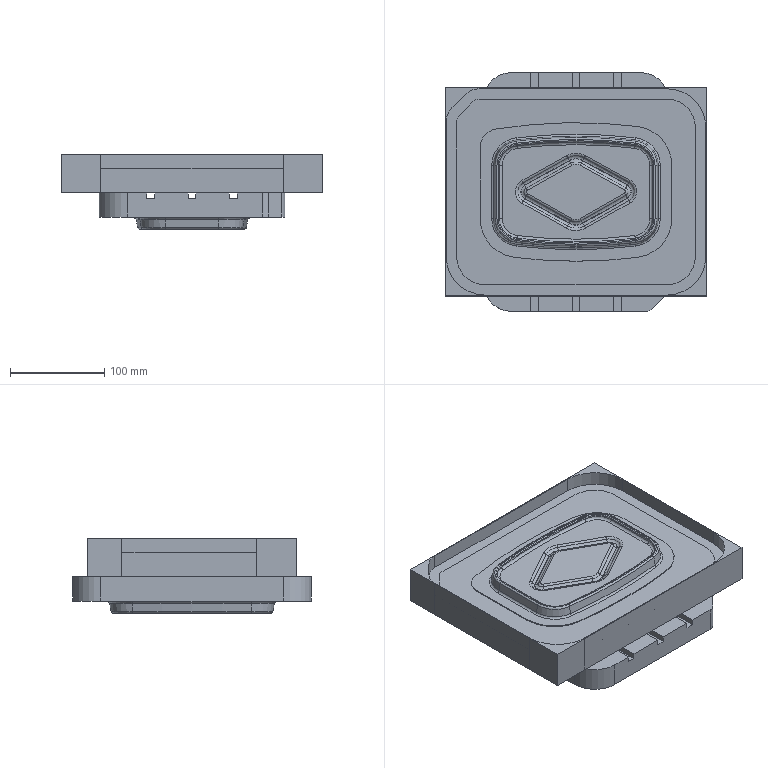NC program | NX | posted with a generic post | part box 278.144 x 254.144 x 79 mm
Lines 98093 to 98150 of 124328:
(DRILLING , TOOL : V2.0)
N196172 M6
N196174 G53
N196176 G17 G0 G90 X-85.236 Y-49.014 S2000 M3 M8
N196178 G43 Z100.5 H0
N196180 G94 G81 G98 Z24.606 F150. R29.606
N196182 X-92.778 Y-25.395
N196184 Y0.
N196186 Y25.395
N196188 X-85.236 Y49.014
N196190 X-63.335 Y60.56
N196192 X-68. Y44. Z31.98 R36.98
N196194 Y22.
N196196 Y0.
N196198 Y-22.
N196200 Y-44.
N196202 X-63.335 Y-60.56 Z24.606 R29.606
N196204 X-38.06 Y-63.002
N196206 X-34. Y-44. Z31.98 R36.98
N196208 Y-22. Z31.366 R36.366
N196210 Y0. Z31.98 R36.98
N196212 Y22. Z31.387 R36.387
N196214 Y44. Z31.98 R36.98
N196216 X-38.06 Y63.002 Z24.606 R29.606
N196218 X-12.696 Y64.225
N196220 X12.696
N196222 X38.06 Y63.002
N196224 X63.335 Y60.56
N196226 X85.236 Y49.014
N196228 X92.778 Y25.395
N196230 Y0.
N196232 Y-25.395
N196234 X85.236 Y-49.014
N196236 X63.335 Y-60.56
N196238 X68. Y-44. Z31.98 R36.98
N196240 Y-22.
N196242 Y0.
N196244 Y22.
N196246 Y44.
N196248 X34.
N196250 Y22. Z31.207 R36.207
N196252 Y0. Z31.98 R36.98
N196254 Y-22. Z31.518 R36.518
N196256 Y-44. Z31.98 R36.98
N196258 X38.06 Y-63.002 Z24.606 R29.606
N196260 X12.696 Y-64.225
N196262 X-12.696
N196264 X0. Y-44. Z31.98 R36.98
N196266 Y-22.
N196268 Y0.
N196270 Y22.
N196272 Y44.
N196274 G80
N196276 G0 X0. Y44. Z100.5
N196278 M9
N196280 M5